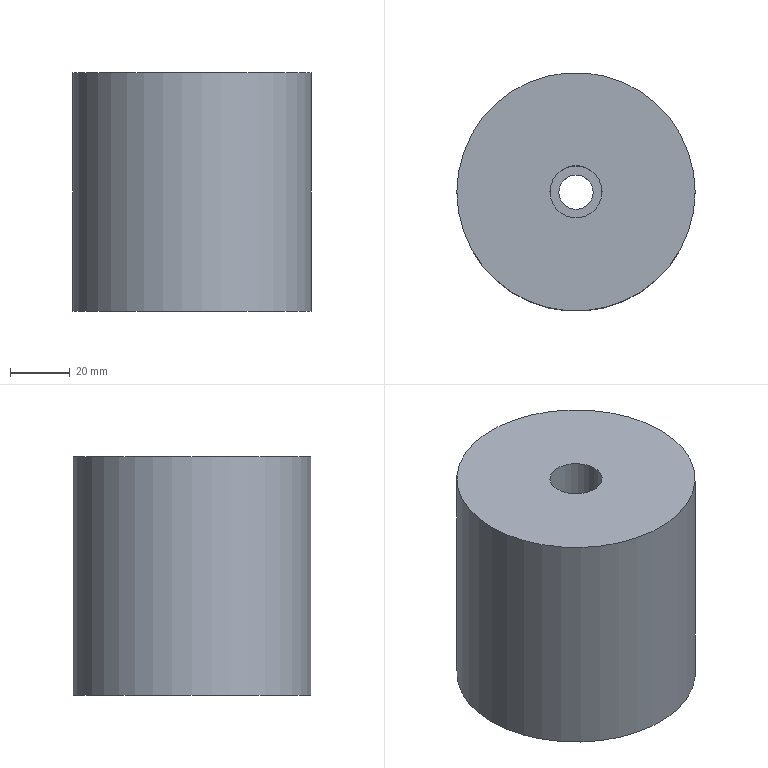Part | NX | features solid 2 | 1 solid | 6 faces | box 80 x 80 x 80 mm | volume 385615 mm3 | plane 3 | cylinder 3 | commonest cylinder face diameters 11.5 x1 17.5 x1 80 x1
STEP:
#1=CARTESIAN_POINT('',(-1213.75,505.,-20.));
#2=VERTEX_POINT('',#1);
#3=CARTESIAN_POINT('',(-1205.,505.,-20.));
#4=DIRECTION('',(0.,0.,-1.));
#5=DIRECTION('',(-1.,0.,0.));
#6=AXIS2_PLACEMENT_3D('',#3,#4,#5);
#7=CIRCLE('',#6,8.75);
#8=EDGE_CURVE('',#2,#2,#7,.T.);
#9=ORIENTED_EDGE('',*,*,#8,.T.);
#10=EDGE_LOOP('',(#9));
#11=FACE_BOUND('',#10,.T.);
#12=CARTESIAN_POINT('',(-1245.,505.,-20.));
#13=VERTEX_POINT('',#12);
#14=CARTESIAN_POINT('',(-1205.,505.,-20.));
#15=DIRECTION('',(0.,0.,-1.));
#16=DIRECTION('',(-1.,0.,0.));
#17=AXIS2_PLACEMENT_3D('',#14,#15,#16);
#18=CIRCLE('',#17,40.);
#19=EDGE_CURVE('',#13,#13,#18,.T.);
#20=ORIENTED_EDGE('',*,*,#19,.F.);
#21=EDGE_LOOP('',(#20));
#22=FACE_BOUND('',#21,.T.);
#23=CARTESIAN_POINT('',(-1205.,505.,-20.));
#24=DIRECTION('',(0.,0.,1.));
#25=DIRECTION('',(-1.,0.,0.));
#26=AXIS2_PLACEMENT_3D('',#23,#24,#25);
#27=PLANE('',#26);
#28=ADVANCED_FACE('',(#11,#22),#27,.T.);
#29=CARTESIAN_POINT('',(-1245.,505.,-100.));
#30=VERTEX_POINT('',#29);
#31=CARTESIAN_POINT('',(-1205.,505.,-100.));
#32=DIRECTION('',(0.,0.,-1.));
#33=DIRECTION('',(-1.,0.,0.));
#34=AXIS2_PLACEMENT_3D('',#31,#32,#33);
#35=CIRCLE('',#34,40.);
#36=EDGE_CURVE('',#30,#30,#35,.T.);
#37=ORIENTED_EDGE('',*,*,#36,.T.);
#38=EDGE_LOOP('',(#37));
#39=FACE_BOUND('',#38,.T.);
#40=CARTESIAN_POINT('',(-1210.75,505.,-100.));
#41=VERTEX_POINT('',#40);
#42=CARTESIAN_POINT('',(-1205.,505.,-100.));
#43=DIRECTION('',(0.,0.,-1.));
#44=DIRECTION('',(-1.,0.,0.));
#45=AXIS2_PLACEMENT_3D('',#42,#43,#44);
#46=CIRCLE('',#45,5.75);
#47=EDGE_CURVE('',#41,#41,#46,.T.);
#48=ORIENTED_EDGE('',*,*,#47,.F.);
#49=EDGE_LOOP('',(#48));
#50=FACE_BOUND('',#49,.T.);
#51=CARTESIAN_POINT('',(-1205.,505.,-100.));
#52=DIRECTION('',(0.,0.,1.));
#53=DIRECTION('',(-1.,0.,0.));
#54=AXIS2_PLACEMENT_3D('',#51,#52,#53);
#55=PLANE('',#54);
#56=ADVANCED_FACE('',(#39,#50),#55,.F.);
#57=CARTESIAN_POINT('',(-1213.75,505.,-80.));
#58=VERTEX_POINT('',#57);
#59=CARTESIAN_POINT('',(-1205.,505.,-80.));
#60=DIRECTION('',(0.,0.,-1.));
#61=DIRECTION('',(-1.,0.,0.));
#62=AXIS2_PLACEMENT_3D('',#59,#60,#61);
#63=CIRCLE('',#62,8.75);
#64=EDGE_CURVE('',#58,#58,#63,.T.);
#65=ORIENTED_EDGE('',*,*,#64,.F.);
#66=EDGE_LOOP('',(#65));
#67=FACE_BOUND('',#66,.T.);
#68=CARTESIAN_POINT('',(-1210.75,505.,-80.));
#69=VERTEX_POINT('',#68);
#70=CARTESIAN_POINT('',(-1205.,505.,-80.));
#71=DIRECTION('',(0.,0.,-1.));
#72=DIRECTION('',(-1.,0.,0.));
#73=AXIS2_PLACEMENT_3D('',#70,#71,#72);
#74=CIRCLE('',#73,5.75);
#75=EDGE_CURVE('',#69,#69,#74,.T.);
#76=ORIENTED_EDGE('',*,*,#75,.T.);
#77=EDGE_LOOP('',(#76));
#78=FACE_BOUND('',#77,.T.);
#79=CARTESIAN_POINT('',(-1205.,505.,-80.));
#80=DIRECTION('',(0.,0.,1.));
#81=DIRECTION('',(-1.,0.,0.));
#82=AXIS2_PLACEMENT_3D('',#79,#80,#81);
#83=PLANE('',#82);
#84=ADVANCED_FACE('',(#67,#78),#83,.T.);
#85=ORIENTED_EDGE('',*,*,#19,.T.);
#86=EDGE_LOOP('',(#85));
#87=FACE_BOUND('',#86,.T.);
#88=ORIENTED_EDGE('',*,*,#36,.F.);
#89=EDGE_LOOP('',(#88));
#90=FACE_BOUND('',#89,.T.);
#91=CARTESIAN_POINT('',(-1205.,505.,0.));
#92=DIRECTION('',(0.,0.,-1.));
#93=DIRECTION('',(1.,0.,0.));
#94=AXIS2_PLACEMENT_3D('',#91,#92,#93);
#95=CYLINDRICAL_SURFACE('',#94,40.);
#96=ADVANCED_FACE('',(#87,#90),#95,.T.);
#97=ORIENTED_EDGE('',*,*,#8,.F.);
#98=EDGE_LOOP('',(#97));
#99=FACE_BOUND('',#98,.T.);
#100=ORIENTED_EDGE('',*,*,#64,.T.);
#101=EDGE_LOOP('',(#100));
#102=FACE_BOUND('',#101,.T.);
#103=CARTESIAN_POINT('',(-1205.,505.,0.));
#104=DIRECTION('',(0.,0.,-1.));
#105=DIRECTION('',(1.,0.,0.));
#106=AXIS2_PLACEMENT_3D('',#103,#104,#105);
#107=CYLINDRICAL_SURFACE('',#106,8.75);
#108=ADVANCED_FACE('',(#99,#102),#107,.F.);
#109=ORIENTED_EDGE('',*,*,#75,.F.);
#110=EDGE_LOOP('',(#109));
#111=FACE_BOUND('',#110,.T.);
#112=ORIENTED_EDGE('',*,*,#47,.T.);
#113=EDGE_LOOP('',(#112));
#114=FACE_BOUND('',#113,.T.);
#115=CARTESIAN_POINT('',(-1205.,505.,-80.));
#116=DIRECTION('',(0.,0.,-1.));
#117=DIRECTION('',(1.,0.,0.));
#118=AXIS2_PLACEMENT_3D('',#115,#116,#117);
#119=CYLINDRICAL_SURFACE('',#118,5.75);
#120=ADVANCED_FACE('',(#111,#114),#119,.F.);
#121=CLOSED_SHELL('',(#28,#56,#84,#96,#108,#120));
#122=MANIFOLD_SOLID_BREP('',#121);
#123=(LENGTH_UNIT()NAMED_UNIT(*)SI_UNIT(.MILLI.,.METRE.));
#124=UNCERTAINTY_MEASURE_WITH_UNIT(LENGTH_MEASURE(0.00001),#123,'','');
#125=(NAMED_UNIT(*)PLANE_ANGLE_UNIT()SI_UNIT($,.RADIAN.));
#126=(NAMED_UNIT(*)SI_UNIT($,.STERADIAN.)SOLID_ANGLE_UNIT());
#127=(GEOMETRIC_REPRESENTATION_CONTEXT(3)GLOBAL_UNCERTAINTY_ASSIGNED_CONTEXT((#124))GLOBAL_UNIT_ASSIGNED_CONTEXT((#123,#125,#126))REPRESENTATION_CONTEXT('',''));
#128=ADVANCED_BREP_SHAPE_REPRESENTATION('',(#122),#127);